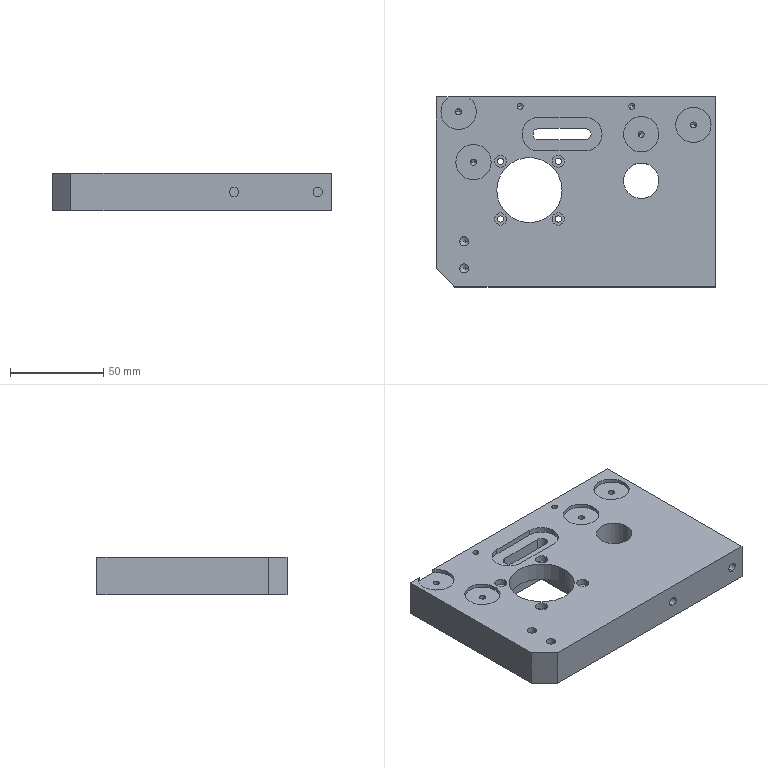Part | STEP file | Front rail (right) | 1 solid | 116 faces | box 150 x 102 x 20 mm | volume 257499 mm3 | cylinder 64 | plane 30 | cone 22 | commonest cylinder face diameters 3.3 x12 19 x11 3.4 x8 5 x8 6.5 x8 4.2 x6